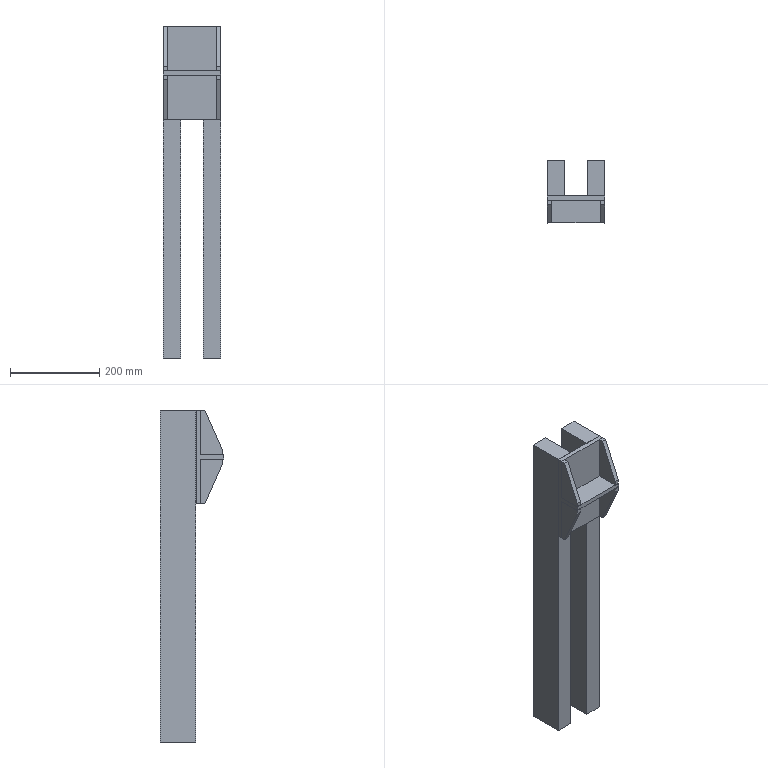Part | STEP file | Connecting plate | 7 solids | 52 faces | box 130 x 142.1 x 745 mm | volume 5233440 mm3 | plane 52